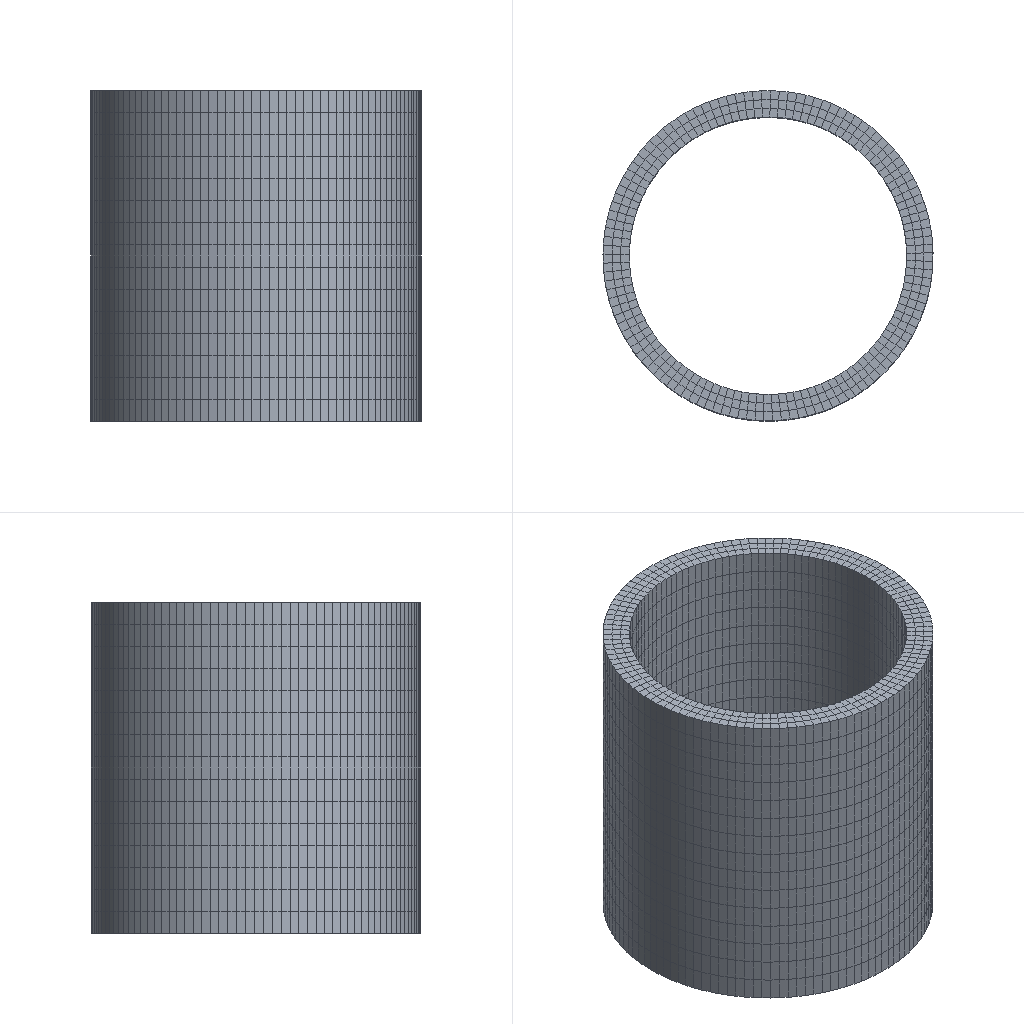Simulation study | abaqus
Set-up summary:
category,name,step,type,value,unit,region
solver,abaqus
solver,version,,,Abaqus/Standard 2020
units,not stated in the deck,,not stated
analysis,deck,,direct cyclic,direct cyclic
load_step,Step-1,Step-1,direct cyclic
load_step,requested,,,1
mesh,nodes,,,7552
mesh,elements,,,5310
element_type,C3D8R,,solid,5310
load,load commands in deck,,count,1
bc,support commands in deck,,count,3
material,MATERIAL-1,,in results
check,setup vs results,,match,"per instance, exact: element labels, types and connectivity; labels of the nodes the elements use; coordinates of those nodes at SINGLE_PRECISION in 1 of 1 instance(s)"
Abaqus input file, long lists of numbers shortened:
*Heading
** Job name: Job-1 Model name: Model-1
** Generated by: Abaqus/CAE 2020
*Preprint, echo=NO, model=NO, history=NO, contact=NO
**
** PARTS
**
*Part, name=Part-1
*Node
      1,   194.333,   247.91,           0.
      2,   231.464,   295.041,           0.
** (7550 more lines like these left out)
*Element, type=C3D8R
   1,  473,  484,  719,  553,    1,   12,  247,   81
   2,  484,  485,  720,  719,   12,   13,  248,  247
** (5308 more lines like these left out)
*Nset, nset=Set-3, generate
    1,  7552,     1
*Elset, elset=Set-3, generate
    1,  5310,     1
** Section: Section-1
*Solid Section, elset=Set-3, material=Material-1
,
*End Part
**
*Part, name=caarck
*End Part
**
**
** ASSEMBLY
**
*Assembly, name=Assembly
**
*Instance, name=Part-1-1, part=Part-1
*End Instance
**
*Instance, name=caarck-1, part=caarck
 -306.841, -247.144, 372.941
 -306.841, -247.144, 372.941, -306.97, -247.015, 373.924, 90.976
*End Instance
**
*Nset, nset=Set-1, instance=Part-1-1
    1,    2,    3,    4,    5,    6,    7,    8,    9,   10,   11,   12,   13,   14,   15,   16
   17,   18,   19,   20,   21,   22,   23,   24,   25,   26,   27,   28,   29,   30,   31,   32
** (57 more lines like these left out)
*Elset, elset=Set-1, instance=Part-1-1
    1,    2,    3,    4,    5,    6,    7,    8,    9,   10,   11,   12,   13,   14,   15,   16
   17,   18,   19,   20,   21,   22,   23,   24,   25,   26,   27,   28,   29,   30,   31,   32
** (43 more lines like these left out)
*Nset, nset=_PickedSet11, internal, instance=Part-1-1, generate
    1,  7552,     1
*Elset, elset=_PickedSet11, internal, instance=Part-1-1, generate
    1,  5310,     1
*Elset, elset=_Surf-1_S6, internal, instance=Part-1-1
    1,    4,    7,   10,   13,   16,   19,   22,   25,   28,   31,   34,   37,   40,   43,   46
   49,   52,   55,   58,   61,   64,   67,   70,   73,   76,   79,   82,   85,   88,   91,   94
** (49 more lines like these left out)
*Elset, elset=_Surf-1_S4, internal, instance=Part-1-1
  105,  108,  111,  114,  117,  120,  123,  126,  129,  132,  135,  138,  141,  144,  147,  150
  153,  156,  159,  162,  165,  168,  171,  174,  177,  180,  183,  186,  189,  192,  195,  198
** (58 more lines like these left out)
*Surface, type=ELEMENT, name=Surf-1
_Surf-1_S6, S6
_Surf-1_S4, S4
*Enrichment, name=Crack-1, type=PROPAGATION CRACK, elset=_PickedSet11, interaction=IntProp-1
*End Assembly
*Amplitude, name=Amp-1, definition=PERIODIC
1,            296.,              0.,              0.
             1.,              0.
**
** MATERIALS
**
*Material, name=Material-1
*Elastic
72000., 0.3
**
** INTERACTION PROPERTIES
**
*Surface Interaction, name=IntProp-1
1.,
*Fracture Criterion,type=FATIGUE,mixed mode behavior=POWER
0.05,-0.1,0.000023,1,0.004,0.7,0.3,0.5,
0.5,0.1,0.2,0.3
*Initial Conditions, type=ENRICHMENT
Part-1-1.263, 1,Crack-1, 36.19, -13.995
Part-1-1.263, 2,Crack-1, 39.132, 3.381
Part-1-1.263, 3,Crack-1, 35.148, 2.909
Part-1-1.263, 4,Crack-1, 31.967, -13.445
Part-1-1.263, 5,Crack-1, -12.107, 0.
Part-1-1.263, 6,Crack-1, -9.164, 14.983
Part-1-1.263, 7,Crack-1, -13.149, 2.909
Part-1-1.263, 8,Crack-1, -16.329, -11.41
Part-1-1.263, 1,Crack-1, 31.967, -13.445
Part-1-1.263, 2,Crack-1, 35.148, 2.909
Part-1-1.263, 3,Crack-1, 31.324, 14.585
Part-1-1.263, 4,Crack-1, 27.915, -1.072
Part-1-1.263, 5,Crack-1, -16.329, -11.41
Part-1-1.263, 6,Crack-1, -13.149, 2.909
Part-1-1.263, 7,Crack-1, -16.973, 14.585
Part-1-1.263, 8,Crack-1, -20.381, -1.072
Part-1-1.263, 1,Crack-1, 27.915, -1.072
Part-1-1.263, 2,Crack-1, 31.324, 14.585
Part-1-1.263, 3,Crack-1, 27.667, 27.023
Part-1-1.263, 4,Crack-1, 24.041, 12.111
Part-1-1.263, 5,Crack-1, -20.381, -1.072
Part-1-1.263, 6,Crack-1, -16.973, 14.585
Part-1-1.263, 7,Crack-1, -20.629, 27.022
Part-1-1.263, 8,Crack-1, -24.255, 12.11
** ----------------------------------------------------------------
**
** STEP: Step-1
**
*Step, name=Step-1, nlgeom=NO, inc=100000
*Direct Cyclic, continue=NO, fatigue
0.01, 1., , , 25, , , 5
1, 3, 10,
**
** BOUNDARY CONDITIONS
**
** Name: BC-1 Type: 位移/转角
*Boundary, amplitude=Amp-1
Set-1, 3, 3
Set-1, 4, 4
Set-1, 5, 5
**
** LOADS
**
** Name: Load-1   Type: Pressure
*Dsload, amplitude=Amp-1
Surf-1, P, 10.
**
** OUTPUT REQUESTS
**
*Restart, write, frequency=0
**
** FIELD OUTPUT: F-Output-1
**
*Output, field
*Node Output
CF, PHILSM, PSILSM, RF, U
*Element Output, directions=YES
E, ENRRTXFEM, LE, LOADSXFEM, MISES, PE, PEEQ, PEMAG, S, SDEG, STATUS, STATUSXFEM
*Contact Output
CDISP, CSTRESS
**
** HISTORY OUTPUT: H-Output-1
**
*Output, history, variable=PRESELECT
*End Step
Results summary:
result,step,,partial,increments=0 time=0.0/1.0
result,analysis,,,static
result,last_loadstep,,,1
result,primary field,,,U
result,reaction total,,FX,0.0,model units
result,reaction total,,FY,0.0,model units
result,reaction total,,FZ,-0.002015,model units